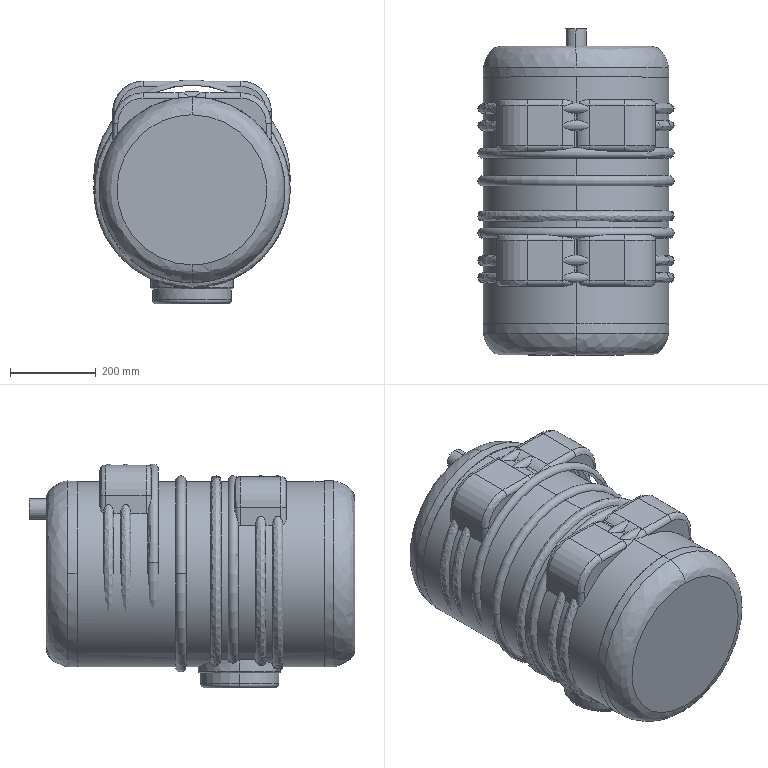Part | SolidWorks | features BaseBody 3, Fillet 2, ICE 2, Scale 1 | 3 solids | 128 faces | box 457.649 x 760 x 522.429 mm | volume 110606732 mm3 | cylinder 61 | plane 26 | torus 21 | spline 20 | commonest cylinder face diameters 433.648 x17 24.8 x16 90.544 x12 142.464 x4 40 x2 48 x2